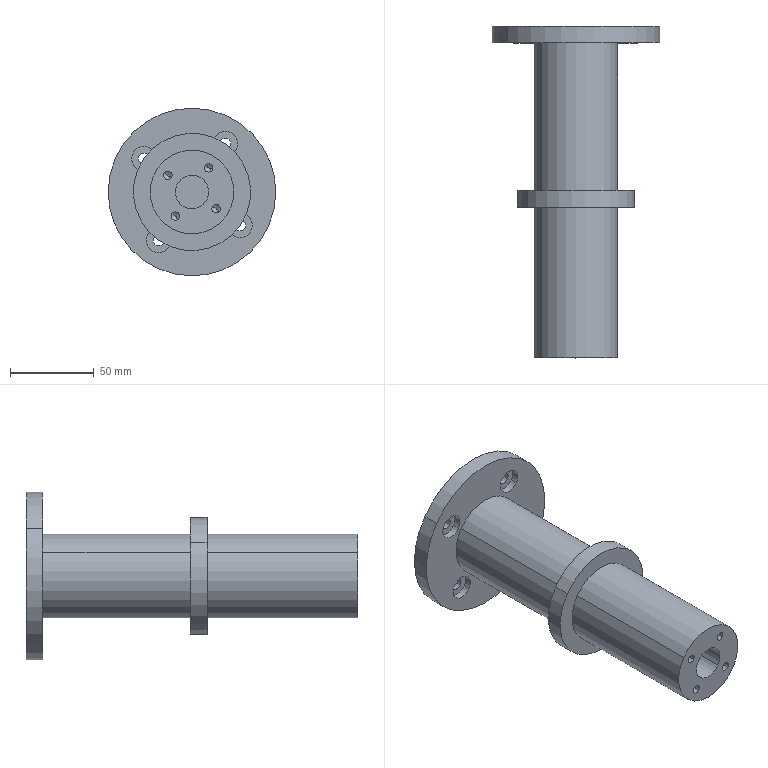Part | STEP file | M6 Tapped Hole 1 | 1 solid | 52 faces | box 100 x 198 x 100 mm | volume 452324 mm3 | cylinder 34 | plane 10 | cone 8 | commonest cylinder face diameters 5 x8 6.6 x8 14.55 x8 50 x4 20 x2 70 x2
STEP:
#1=CARTESIAN_POINT('',(-1578.988,1475.264,2948.123));
#2=VERTEX_POINT('',#1);
#3=CARTESIAN_POINT('',(-1574.875,1475.264,2945.28));
#4=VERTEX_POINT('',#3);
#5=CARTESIAN_POINT('',(-1576.931,1475.264,2946.701));
#6=DIRECTION('',(0.,-1.,0.));
#7=DIRECTION('',(0.8226,0.,-0.5686));
#8=AXIS2_PLACEMENT_3D('',#5,#6,#7);
#9=CIRCLE('',#8,2.5);
#10=EDGE_CURVE('',#2,#4,#9,.T.);
#11=ORIENTED_EDGE('',*,*,#10,.F.);
#12=CARTESIAN_POINT('',(-1578.988,1460.264,2948.123));
#13=VERTEX_POINT('',#12);
#14=CARTESIAN_POINT('',(-1578.988,1460.264,2948.123));
#15=DIRECTION('',(0.,1.,0.));
#16=VECTOR('',#15,1000.);
#17=LINE('',#14,#16);
#18=EDGE_CURVE('',#13,#2,#17,.T.);
#19=ORIENTED_EDGE('',*,*,#18,.F.);
#20=CARTESIAN_POINT('',(-1574.875,1460.264,2945.28));
#21=VERTEX_POINT('',#20);
#22=CARTESIAN_POINT('',(-1576.931,1460.264,2946.701));
#23=DIRECTION('',(0.,-1.,0.));
#24=DIRECTION('',(0.8226,0.,-0.5686));
#25=AXIS2_PLACEMENT_3D('',#22,#23,#24);
#26=CIRCLE('',#25,2.5);
#27=EDGE_CURVE('',#13,#21,#26,.T.);
#28=ORIENTED_EDGE('',*,*,#27,.T.);
#29=CARTESIAN_POINT('',(-1574.875,1460.264,2945.28));
#30=DIRECTION('',(0.,1.,0.));
#31=VECTOR('',#30,1000.);
#32=LINE('',#29,#31);
#33=EDGE_CURVE('',#21,#4,#32,.T.);
#34=ORIENTED_EDGE('',*,*,#33,.T.);
#35=EDGE_LOOP('',(#11,#19,#28,#34));
#36=FACE_OUTER_BOUND('',#35,.T.);
#37=CARTESIAN_POINT('',(-1576.931,1460.264,2946.701));
#38=DIRECTION('',(0.,-1.,0.));
#39=DIRECTION('',(-0.8226,0.,0.5686));
#40=AXIS2_PLACEMENT_3D('',#37,#38,#39);
#41=CYLINDRICAL_SURFACE('',#40,2.5);
#42=ADVANCED_FACE('',(#36),#41,.F.);
#43=CARTESIAN_POINT('',(-1576.931,1476.766,2946.701));
#44=VERTEX_POINT('',#43);
#45=CARTESIAN_POINT('',(-1574.875,1475.264,2945.28));
#46=DIRECTION('',(-0.7051,0.515,0.4874));
#47=VECTOR('',#46,1000.);
#48=LINE('',#45,#47);
#49=EDGE_CURVE('',#4,#44,#48,.T.);
#50=ORIENTED_EDGE('',*,*,#49,.T.);
#51=CARTESIAN_POINT('',(-1578.988,1475.264,2948.123));
#52=DIRECTION('',(0.7051,0.515,-0.4874));
#53=VECTOR('',#52,1000.);
#54=LINE('',#51,#53);
#55=EDGE_CURVE('',#2,#44,#54,.T.);
#56=ORIENTED_EDGE('',*,*,#55,.F.);
#57=ORIENTED_EDGE('',*,*,#10,.T.);
#58=EDGE_LOOP('',(#50,#56,#57));
#59=FACE_OUTER_BOUND('',#58,.T.);
#60=CARTESIAN_POINT('',(-1576.931,1475.264,2946.701));
#61=DIRECTION('',(0.,-1.,0.));
#62=DIRECTION('',(-0.8226,0.,0.5686));
#63=AXIS2_PLACEMENT_3D('',#60,#61,#62);
#64=CONICAL_SURFACE('',#63,2.5,1.03);
#65=ADVANCED_FACE('',(#59),#64,.F.);
#66=CARTESIAN_POINT('',(-1554.641,1475.264,2952.568));
#67=VERTEX_POINT('',#66);
#68=CARTESIAN_POINT('',(-1550.528,1475.264,2949.725));
#69=VERTEX_POINT('',#68);
#70=CARTESIAN_POINT('',(-1552.585,1475.264,2951.146));
#71=DIRECTION('',(0.,-1.,0.));
#72=DIRECTION('',(0.8226,0.,-0.5686));
#73=AXIS2_PLACEMENT_3D('',#70,#71,#72);
#74=CIRCLE('',#73,2.5);
#75=EDGE_CURVE('',#67,#69,#74,.T.);
#76=ORIENTED_EDGE('',*,*,#75,.F.);
#77=CARTESIAN_POINT('',(-1554.641,1460.264,2952.568));
#78=VERTEX_POINT('',#77);
#79=CARTESIAN_POINT('',(-1554.641,1460.264,2952.568));
#80=DIRECTION('',(0.,1.,0.));
#81=VECTOR('',#80,1000.);
#82=LINE('',#79,#81);
#83=EDGE_CURVE('',#78,#67,#82,.T.);
#84=ORIENTED_EDGE('',*,*,#83,.F.);
#85=CARTESIAN_POINT('',(-1550.528,1460.264,2949.725));
#86=VERTEX_POINT('',#85);
#87=CARTESIAN_POINT('',(-1552.585,1460.264,2951.146));
#88=DIRECTION('',(0.,-1.,0.));
#89=DIRECTION('',(0.8226,0.,-0.5686));
#90=AXIS2_PLACEMENT_3D('',#87,#88,#89);
#91=CIRCLE('',#90,2.5);
#92=EDGE_CURVE('',#78,#86,#91,.T.);
#93=ORIENTED_EDGE('',*,*,#92,.T.);
#94=CARTESIAN_POINT('',(-1550.528,1460.264,2949.725));
#95=DIRECTION('',(0.,1.,0.));
#96=VECTOR('',#95,1000.);
#97=LINE('',#94,#96);
#98=EDGE_CURVE('',#86,#69,#97,.T.);
#99=ORIENTED_EDGE('',*,*,#98,.T.);
#100=EDGE_LOOP('',(#76,#84,#93,#99));
#101=FACE_OUTER_BOUND('',#100,.T.);
#102=CARTESIAN_POINT('',(-1552.585,1460.264,2951.146));
#103=DIRECTION('',(0.,-1.,0.));
#104=DIRECTION('',(-0.8226,0.,0.5686));
#105=AXIS2_PLACEMENT_3D('',#102,#103,#104);
#106=CYLINDRICAL_SURFACE('',#105,2.5);
#107=ADVANCED_FACE('',(#101),#106,.F.);
#108=CARTESIAN_POINT('',(-1552.585,1476.766,2951.146));
#109=VERTEX_POINT('',#108);
#110=CARTESIAN_POINT('',(-1550.528,1475.264,2949.725));
#111=DIRECTION('',(-0.7051,0.515,0.4874));
#112=VECTOR('',#111,1000.);
#113=LINE('',#110,#112);
#114=EDGE_CURVE('',#69,#109,#113,.T.);
#115=ORIENTED_EDGE('',*,*,#114,.T.);
#116=CARTESIAN_POINT('',(-1554.641,1475.264,2952.568));
#117=DIRECTION('',(0.7051,0.515,-0.4874));
#118=VECTOR('',#117,1000.);
#119=LINE('',#116,#118);
#120=EDGE_CURVE('',#67,#109,#119,.T.);
#121=ORIENTED_EDGE('',*,*,#120,.F.);
#122=ORIENTED_EDGE('',*,*,#75,.T.);
#123=EDGE_LOOP('',(#115,#121,#122));
#124=FACE_OUTER_BOUND('',#123,.T.);
#125=CARTESIAN_POINT('',(-1552.585,1475.264,2951.146));
#126=DIRECTION('',(0.,-1.,0.));
#127=DIRECTION('',(-0.8226,0.,0.5686));
#128=AXIS2_PLACEMENT_3D('',#125,#126,#127);
#129=CONICAL_SURFACE('',#128,2.5,1.03);
#130=ADVANCED_FACE('',(#124),#129,.F.);
#131=CARTESIAN_POINT('',(-1550.196,1475.264,2928.222));
#132=VERTEX_POINT('',#131);
#133=CARTESIAN_POINT('',(-1546.083,1475.264,2925.378));
#134=VERTEX_POINT('',#133);
#135=CARTESIAN_POINT('',(-1548.14,1475.264,2926.8));
#136=DIRECTION('',(0.,-1.,0.));
#137=DIRECTION('',(0.8226,0.,-0.5686));
#138=AXIS2_PLACEMENT_3D('',#135,#136,#137);
#139=CIRCLE('',#138,2.5);
#140=EDGE_CURVE('',#132,#134,#139,.T.);
#141=ORIENTED_EDGE('',*,*,#140,.F.);
#142=CARTESIAN_POINT('',(-1550.196,1460.264,2928.222));
#143=VERTEX_POINT('',#142);
#144=CARTESIAN_POINT('',(-1550.196,1460.264,2928.222));
#145=DIRECTION('',(0.,1.,0.));
#146=VECTOR('',#145,1000.);
#147=LINE('',#144,#146);
#148=EDGE_CURVE('',#143,#132,#147,.T.);
#149=ORIENTED_EDGE('',*,*,#148,.F.);
#150=CARTESIAN_POINT('',(-1546.083,1460.264,2925.378));
#151=VERTEX_POINT('',#150);
#152=CARTESIAN_POINT('',(-1548.14,1460.264,2926.8));
#153=DIRECTION('',(0.,-1.,0.));
#154=DIRECTION('',(0.8226,0.,-0.5686));
#155=AXIS2_PLACEMENT_3D('',#152,#153,#154);
#156=CIRCLE('',#155,2.5);
#157=EDGE_CURVE('',#143,#151,#156,.T.);
#158=ORIENTED_EDGE('',*,*,#157,.T.);
#159=CARTESIAN_POINT('',(-1546.083,1460.264,2925.378));
#160=DIRECTION('',(0.,1.,0.));
#161=VECTOR('',#160,1000.);
#162=LINE('',#159,#161);
#163=EDGE_CURVE('',#151,#134,#162,.T.);
#164=ORIENTED_EDGE('',*,*,#163,.T.);
#165=EDGE_LOOP('',(#141,#149,#158,#164));
#166=FACE_OUTER_BOUND('',#165,.T.);
#167=CARTESIAN_POINT('',(-1548.14,1460.264,2926.8));
#168=DIRECTION('',(0.,-1.,0.));
#169=DIRECTION('',(-0.8226,0.,0.5686));
#170=AXIS2_PLACEMENT_3D('',#167,#168,#169);
#171=CYLINDRICAL_SURFACE('',#170,2.5);
#172=ADVANCED_FACE('',(#166),#171,.F.);
#173=CARTESIAN_POINT('',(-1548.14,1476.766,2926.8));
#174=VERTEX_POINT('',#173);
#175=CARTESIAN_POINT('',(-1546.083,1475.264,2925.378));
#176=DIRECTION('',(-0.7051,0.515,0.4874));
#177=VECTOR('',#176,1000.);
#178=LINE('',#175,#177);
#179=EDGE_CURVE('',#134,#174,#178,.T.);
#180=ORIENTED_EDGE('',*,*,#179,.T.);
#181=CARTESIAN_POINT('',(-1550.196,1475.264,2928.222));
#182=DIRECTION('',(0.7051,0.515,-0.4874));
#183=VECTOR('',#182,1000.);
#184=LINE('',#181,#183);
#185=EDGE_CURVE('',#132,#174,#184,.T.);
#186=ORIENTED_EDGE('',*,*,#185,.F.);
#187=ORIENTED_EDGE('',*,*,#140,.T.);
#188=EDGE_LOOP('',(#180,#186,#187));
#189=FACE_OUTER_BOUND('',#188,.T.);
#190=CARTESIAN_POINT('',(-1548.14,1475.264,2926.8));
#191=DIRECTION('',(0.,-1.,0.));
#192=DIRECTION('',(-0.8226,0.,0.5686));
#193=AXIS2_PLACEMENT_3D('',#190,#191,#192);
#194=CONICAL_SURFACE('',#193,2.5,1.03);
#195=ADVANCED_FACE('',(#189),#194,.F.);
#196=CARTESIAN_POINT('',(-1574.543,1475.264,2923.777));
#197=VERTEX_POINT('',#196);
#198=CARTESIAN_POINT('',(-1570.43,1475.264,2920.934));
#199=VERTEX_POINT('',#198);
#200=CARTESIAN_POINT('',(-1572.486,1475.264,2922.355));
#201=DIRECTION('',(0.,-1.,0.));
#202=DIRECTION('',(0.8226,0.,-0.5686));
#203=AXIS2_PLACEMENT_3D('',#200,#201,#202);
#204=CIRCLE('',#203,2.5);
#205=EDGE_CURVE('',#197,#199,#204,.T.);
#206=ORIENTED_EDGE('',*,*,#205,.F.);
#207=CARTESIAN_POINT('',(-1574.543,1460.264,2923.777));
#208=VERTEX_POINT('',#207);
#209=CARTESIAN_POINT('',(-1574.543,1460.264,2923.777));
#210=DIRECTION('',(0.,1.,0.));
#211=VECTOR('',#210,1000.);
#212=LINE('',#209,#211);
#213=EDGE_CURVE('',#208,#197,#212,.T.);
#214=ORIENTED_EDGE('',*,*,#213,.F.);
#215=CARTESIAN_POINT('',(-1570.43,1460.264,2920.934));
#216=VERTEX_POINT('',#215);
#217=CARTESIAN_POINT('',(-1572.486,1460.264,2922.355));
#218=DIRECTION('',(0.,-1.,0.));
#219=DIRECTION('',(0.8226,0.,-0.5686));
#220=AXIS2_PLACEMENT_3D('',#217,#218,#219);
#221=CIRCLE('',#220,2.5);
#222=EDGE_CURVE('',#208,#216,#221,.T.);
#223=ORIENTED_EDGE('',*,*,#222,.T.);
#224=CARTESIAN_POINT('',(-1570.43,1460.264,2920.934));
#225=DIRECTION('',(0.,1.,0.));
#226=VECTOR('',#225,1000.);
#227=LINE('',#224,#226);
#228=EDGE_CURVE('',#216,#199,#227,.T.);
#229=ORIENTED_EDGE('',*,*,#228,.T.);
#230=EDGE_LOOP('',(#206,#214,#223,#229));
#231=FACE_OUTER_BOUND('',#230,.T.);
#232=CARTESIAN_POINT('',(-1572.486,1460.264,2922.355));
#233=DIRECTION('',(0.,-1.,0.));
#234=DIRECTION('',(-0.8226,0.,0.5686));
#235=AXIS2_PLACEMENT_3D('',#232,#233,#234);
#236=CYLINDRICAL_SURFACE('',#235,2.5);
#237=ADVANCED_FACE('',(#231),#236,.F.);
#238=CARTESIAN_POINT('',(-1572.486,1476.766,2922.355));
#239=VERTEX_POINT('',#238);
#240=CARTESIAN_POINT('',(-1570.43,1475.264,2920.934));
#241=DIRECTION('',(-0.7051,0.515,0.4874));
#242=VECTOR('',#241,1000.);
#243=LINE('',#240,#242);
#244=EDGE_CURVE('',#199,#239,#243,.T.);
#245=ORIENTED_EDGE('',*,*,#244,.T.);
#246=CARTESIAN_POINT('',(-1574.543,1475.264,2923.777));
#247=DIRECTION('',(0.7051,0.515,-0.4874));
#248=VECTOR('',#247,1000.);
#249=LINE('',#246,#248);
#250=EDGE_CURVE('',#197,#239,#249,.T.);
#251=ORIENTED_EDGE('',*,*,#250,.F.);
#252=ORIENTED_EDGE('',*,*,#205,.T.);
#253=EDGE_LOOP('',(#245,#251,#252));
#254=FACE_OUTER_BOUND('',#253,.T.);
#255=CARTESIAN_POINT('',(-1572.486,1475.264,2922.355));
#256=DIRECTION('',(0.,-1.,0.));
#257=DIRECTION('',(-0.8226,0.,0.5686));
#258=AXIS2_PLACEMENT_3D('',#255,#256,#257);
#259=CONICAL_SURFACE('',#258,2.5,1.03);
#260=ADVANCED_FACE('',(#254),#259,.F.);
#261=CARTESIAN_POINT('',(-1570.762,1490.264,2942.437));
#262=VERTEX_POINT('',#261);
#263=CARTESIAN_POINT('',(-1554.309,1490.264,2931.065));
#264=VERTEX_POINT('',#263);
#265=CARTESIAN_POINT('',(-1562.535,1490.264,2936.751));
#266=DIRECTION('',(0.,-1.,0.));
#267=DIRECTION('',(0.8226,0.,-0.5686));
#268=AXIS2_PLACEMENT_3D('',#265,#266,#267);
#269=CIRCLE('',#268,10.);
#270=EDGE_CURVE('',#262,#264,#269,.T.);
#271=ORIENTED_EDGE('',*,*,#270,.F.);
#272=CARTESIAN_POINT('',(-1570.762,1460.264,2942.437));
#273=VERTEX_POINT('',#272);
#274=CARTESIAN_POINT('',(-1570.762,1490.264,2942.437));
#275=DIRECTION('',(0.,1.,0.));
#276=VECTOR('',#275,1000.);
#277=LINE('',#274,#276);
#278=EDGE_CURVE('',#273,#262,#277,.T.);
#279=ORIENTED_EDGE('',*,*,#278,.F.);
#280=CARTESIAN_POINT('',(-1554.309,1460.264,2931.065));
#281=VERTEX_POINT('',#280);
#282=CARTESIAN_POINT('',(-1562.535,1460.264,2936.751));
#283=DIRECTION('',(0.,-1.,0.));
#284=DIRECTION('',(0.8226,0.,-0.5686));
#285=AXIS2_PLACEMENT_3D('',#282,#283,#284);
#286=CIRCLE('',#285,10.);
#287=EDGE_CURVE('',#273,#281,#286,.T.);
#288=ORIENTED_EDGE('',*,*,#287,.T.);
#289=CARTESIAN_POINT('',(-1554.309,1490.264,2931.065));
#290=DIRECTION('',(0.,1.,0.));
#291=VECTOR('',#290,1000.);
#292=LINE('',#289,#291);
#293=EDGE_CURVE('',#281,#264,#292,.T.);
#294=ORIENTED_EDGE('',*,*,#293,.T.);
#295=EDGE_LOOP('',(#271,#279,#288,#294));
#296=FACE_OUTER_BOUND('',#295,.T.);
#297=CARTESIAN_POINT('',(-1562.535,1490.264,2936.751));
#298=DIRECTION('',(0.,-1.,0.));
#299=DIRECTION('',(-0.8226,0.,0.5686));
#300=AXIS2_PLACEMENT_3D('',#297,#298,#299);
#301=CYLINDRICAL_SURFACE('',#300,10.);
#302=ADVANCED_FACE('',(#296),#301,.F.);
#303=CARTESIAN_POINT('',(-1541.97,1550.264,2922.535));
#304=VERTEX_POINT('',#303);
#305=CARTESIAN_POINT('',(-1583.101,1550.264,2950.966));
#306=VERTEX_POINT('',#305);
#307=CARTESIAN_POINT('',(-1562.535,1550.264,2936.751));
#308=DIRECTION('',(0.,-1.,0.));
#309=DIRECTION('',(0.8226,0.,-0.5686));
#310=AXIS2_PLACEMENT_3D('',#307,#308,#309);
#311=CIRCLE('',#310,25.);
#312=EDGE_CURVE('',#304,#306,#311,.T.);
#313=ORIENTED_EDGE('',*,*,#312,.T.);
#314=CARTESIAN_POINT('',(-1583.101,1460.264,2950.966));
#315=VERTEX_POINT('',#314);
#316=CARTESIAN_POINT('',(-1583.101,1648.264,2950.966));
#317=DIRECTION('',(0.,1.,0.));
#318=VECTOR('',#317,1000.);
#319=LINE('',#316,#318);
#320=EDGE_CURVE('',#315,#306,#319,.T.);
#321=ORIENTED_EDGE('',*,*,#320,.F.);
#322=CARTESIAN_POINT('',(-1541.97,1460.264,2922.535));
#323=VERTEX_POINT('',#322);
#324=CARTESIAN_POINT('',(-1562.535,1460.264,2936.751));
#325=DIRECTION('',(0.,1.,0.));
#326=DIRECTION('',(-0.8226,0.,0.5686));
#327=AXIS2_PLACEMENT_3D('',#324,#325,#326);
#328=CIRCLE('',#327,25.);
#329=EDGE_CURVE('',#315,#323,#328,.T.);
#330=ORIENTED_EDGE('',*,*,#329,.T.);
#331=CARTESIAN_POINT('',(-1541.97,1648.264,2922.535));
#332=DIRECTION('',(0.,1.,0.));
#333=VECTOR('',#332,1000.);
#334=LINE('',#331,#333);
#335=EDGE_CURVE('',#323,#304,#334,.T.);
#336=ORIENTED_EDGE('',*,*,#335,.T.);
#337=EDGE_LOOP('',(#313,#321,#330,#336));
#338=FACE_OUTER_BOUND('',#337,.T.);
#339=CARTESIAN_POINT('',(-1562.535,1648.264,2936.751));
#340=DIRECTION('',(0.,-1.,0.));
#341=DIRECTION('',(-0.8226,0.,0.5686));
#342=AXIS2_PLACEMENT_3D('',#339,#340,#341);
#343=CYLINDRICAL_SURFACE('',#342,25.);
#344=ADVANCED_FACE('',(#338),#343,.T.);
#345=CARTESIAN_POINT('',(-1533.744,1550.264,2916.849));
#346=VERTEX_POINT('',#345);
#347=CARTESIAN_POINT('',(-1591.327,1550.264,2956.652));
#348=VERTEX_POINT('',#347);
#349=CARTESIAN_POINT('',(-1562.535,1550.264,2936.751));
#350=DIRECTION('',(0.,-1.,0.));
#351=DIRECTION('',(0.8226,0.,-0.5686));
#352=AXIS2_PLACEMENT_3D('',#349,#350,#351);
#353=CIRCLE('',#352,35.);
#354=EDGE_CURVE('',#346,#348,#353,.T.);
#355=ORIENTED_EDGE('',*,*,#354,.F.);
#356=CARTESIAN_POINT('',(-1533.744,1560.264,2916.849));
#357=VERTEX_POINT('',#356);
#358=CARTESIAN_POINT('',(-1533.744,1550.264,2916.849));
#359=DIRECTION('',(0.,1.,0.));
#360=VECTOR('',#359,1000.);
#361=LINE('',#358,#360);
#362=EDGE_CURVE('',#346,#357,#361,.T.);
#363=ORIENTED_EDGE('',*,*,#362,.T.);
#364=CARTESIAN_POINT('',(-1591.327,1560.264,2956.652));
#365=VERTEX_POINT('',#364);
#366=CARTESIAN_POINT('',(-1562.535,1560.264,2936.751));
#367=DIRECTION('',(0.,-1.,0.));
#368=DIRECTION('',(0.8226,0.,-0.5686));
#369=AXIS2_PLACEMENT_3D('',#366,#367,#368);
#370=CIRCLE('',#369,35.);
#371=EDGE_CURVE('',#357,#365,#370,.T.);
#372=ORIENTED_EDGE('',*,*,#371,.T.);
#373=CARTESIAN_POINT('',(-1591.327,1550.264,2956.652));
#374=DIRECTION('',(0.,1.,0.));
#375=VECTOR('',#374,1000.);
#376=LINE('',#373,#375);
#377=EDGE_CURVE('',#348,#365,#376,.T.);
#378=ORIENTED_EDGE('',*,*,#377,.F.);
#379=EDGE_LOOP('',(#355,#363,#372,#378));
#380=FACE_OUTER_BOUND('',#379,.T.);
#381=CARTESIAN_POINT('',(-1562.535,1550.264,2936.751));
#382=DIRECTION('',(0.,1.,0.));
#383=DIRECTION('',(0.8226,0.,-0.5686));
#384=AXIS2_PLACEMENT_3D('',#381,#382,#383);
#385=CYLINDRICAL_SURFACE('',#384,35.);
#386=ADVANCED_FACE('',(#380),#385,.T.);
#387=CARTESIAN_POINT('',(-1539.729,1652.414,2920.986));
#388=VERTEX_POINT('',#387);
#389=CARTESIAN_POINT('',(-1527.76,1652.414,2912.713));
#390=VERTEX_POINT('',#389);
#391=CARTESIAN_POINT('',(-1533.744,1652.414,2916.849));
#392=DIRECTION('',(0.,-1.,0.));
#393=DIRECTION('',(0.8226,0.,-0.5686));
#394=AXIS2_PLACEMENT_3D('',#391,#392,#393);
#395=CIRCLE('',#394,7.275);
#396=EDGE_CURVE('',#388,#390,#395,.T.);
#397=ORIENTED_EDGE('',*,*,#396,.F.);
#398=CARTESIAN_POINT('',(-1539.729,1648.264,2920.986));
#399=VERTEX_POINT('',#398);
#400=CARTESIAN_POINT('',(-1539.729,1648.264,2920.986));
#401=DIRECTION('',(0.,1.,0.));
#402=VECTOR('',#401,1000.);
#403=LINE('',#400,#402);
#404=EDGE_CURVE('',#399,#388,#403,.T.);
#405=ORIENTED_EDGE('',*,*,#404,.F.);
#406=CARTESIAN_POINT('',(-1527.76,1648.264,2912.713));
#407=VERTEX_POINT('',#406);
#408=CARTESIAN_POINT('',(-1533.744,1648.264,2916.849));
#409=DIRECTION('',(0.,-1.,0.));
#410=DIRECTION('',(0.8226,0.,-0.5686));
#411=AXIS2_PLACEMENT_3D('',#408,#409,#410);
#412=CIRCLE('',#411,7.275);
#413=EDGE_CURVE('',#399,#407,#412,.T.);
#414=ORIENTED_EDGE('',*,*,#413,.T.);
#415=CARTESIAN_POINT('',(-1527.76,1648.264,2912.713));
#416=DIRECTION('',(0.,1.,0.));
#417=VECTOR('',#416,1000.);
#418=LINE('',#415,#417);
#419=EDGE_CURVE('',#407,#390,#418,.T.);
#420=ORIENTED_EDGE('',*,*,#419,.T.);
#421=EDGE_LOOP('',(#397,#405,#414,#420));
#422=FACE_OUTER_BOUND('',#421,.T.);
#423=CARTESIAN_POINT('',(-1533.744,1648.264,2916.849));
#424=DIRECTION('',(0.,-1.,0.));
#425=DIRECTION('',(-0.8226,0.,0.5686));
#426=AXIS2_PLACEMENT_3D('',#423,#424,#425);
#427=CYLINDRICAL_SURFACE('',#426,7.275);
#428=ADVANCED_FACE('',(#422),#427,.F.);
#429=CARTESIAN_POINT('',(-1536.459,1658.264,2918.726));
#430=VERTEX_POINT('',#429);
#431=CARTESIAN_POINT('',(-1531.03,1658.264,2914.973));
#432=VERTEX_POINT('',#431);
#433=CARTESIAN_POINT('',(-1533.744,1658.264,2916.849));
#434=DIRECTION('',(0.,-1.,0.));
#435=DIRECTION('',(0.8226,0.,-0.5686));
#436=AXIS2_PLACEMENT_3D('',#433,#434,#435);
#437=CIRCLE('',#436,3.3);
#438=EDGE_CURVE('',#430,#432,#437,.T.);
#439=ORIENTED_EDGE('',*,*,#438,.F.);
#440=CARTESIAN_POINT('',(-1536.459,1652.414,2918.726));
#441=VERTEX_POINT('',#440);
#442=CARTESIAN_POINT('',(-1536.459,1648.264,2918.726));
#443=DIRECTION('',(0.,1.,0.));
#444=VECTOR('',#443,1000.);
#445=LINE('',#442,#444);
#446=EDGE_CURVE('',#441,#430,#445,.T.);
#447=ORIENTED_EDGE('',*,*,#446,.F.);
#448=CARTESIAN_POINT('',(-1531.03,1652.414,2914.973));
#449=VERTEX_POINT('',#448);
#450=CARTESIAN_POINT('',(-1533.744,1652.414,2916.849));
#451=DIRECTION('',(0.,-1.,0.));
#452=DIRECTION('',(0.8226,0.,-0.5686));
#453=AXIS2_PLACEMENT_3D('',#450,#451,#452);
#454=CIRCLE('',#453,3.3);
#455=EDGE_CURVE('',#441,#449,#454,.T.);
#456=ORIENTED_EDGE('',*,*,#455,.T.);
#457=CARTESIAN_POINT('',(-1531.03,1648.264,2914.973));
#458=DIRECTION('',(0.,1.,0.));
#459=VECTOR('',#458,1000.);
#460=LINE('',#457,#459);
#461=EDGE_CURVE('',#449,#432,#460,.T.);
#462=ORIENTED_EDGE('',*,*,#461,.T.);
#463=EDGE_LOOP('',(#439,#447,#456,#462));
#464=FACE_OUTER_BOUND('',#463,.T.);
#465=CARTESIAN_POINT('',(-1533.744,1648.264,2916.849));
#466=DIRECTION('',(0.,-1.,0.));
#467=DIRECTION('',(-0.8226,0.,0.5686));
#468=AXIS2_PLACEMENT_3D('',#465,#466,#467);
#469=CYLINDRICAL_SURFACE('',#468,3.3);
#470=ADVANCED_FACE('',(#464),#469,.F.);
#471=CARTESIAN_POINT('',(-1588.421,1652.414,2912.096));
#472=VERTEX_POINT('',#471);
#473=CARTESIAN_POINT('',(-1576.452,1652.414,2903.823));
#474=VERTEX_POINT('',#473);
#475=CARTESIAN_POINT('',(-1582.437,1652.414,2907.959));
#476=DIRECTION('',(0.,-1.,0.));
#477=DIRECTION('',(0.8226,0.,-0.5686));
#478=AXIS2_PLACEMENT_3D('',#475,#476,#477);
#479=CIRCLE('',#478,7.275);
#480=EDGE_CURVE('',#472,#474,#479,.T.);
#481=ORIENTED_EDGE('',*,*,#480,.F.);
#482=CARTESIAN_POINT('',(-1588.421,1648.264,2912.096));
#483=VERTEX_POINT('',#482);
#484=CARTESIAN_POINT('',(-1588.421,1648.264,2912.096));
#485=DIRECTION('',(0.,1.,0.));
#486=VECTOR('',#485,1000.);
#487=LINE('',#484,#486);
#488=EDGE_CURVE('',#483,#472,#487,.T.);
#489=ORIENTED_EDGE('',*,*,#488,.F.);
#490=CARTESIAN_POINT('',(-1576.452,1648.264,2903.823));
#491=VERTEX_POINT('',#490);
#492=CARTESIAN_POINT('',(-1582.437,1648.264,2907.959));
#493=DIRECTION('',(0.,-1.,0.));
#494=DIRECTION('',(0.8226,0.,-0.5686));
#495=AXIS2_PLACEMENT_3D('',#492,#493,#494);
#496=CIRCLE('',#495,7.275);
#497=EDGE_CURVE('',#483,#491,#496,.T.);
#498=ORIENTED_EDGE('',*,*,#497,.T.);
#499=CARTESIAN_POINT('',(-1576.452,1648.264,2903.823));
#500=DIRECTION('',(0.,1.,0.));
#501=VECTOR('',#500,1000.);
#502=LINE('',#499,#501);
#503=EDGE_CURVE('',#491,#474,#502,.T.);
#504=ORIENTED_EDGE('',*,*,#503,.T.);
#505=EDGE_LOOP('',(#481,#489,#498,#504));
#506=FACE_OUTER_BOUND('',#505,.T.);
#507=CARTESIAN_POINT('',(-1582.437,1648.264,2907.959));
#508=DIRECTION('',(0.,-1.,0.));
#509=DIRECTION('',(-0.8226,0.,0.5686));
#510=AXIS2_PLACEMENT_3D('',#507,#508,#509);
#511=CYLINDRICAL_SURFACE('',#510,7.275);
#512=ADVANCED_FACE('',(#506),#511,.F.);
#513=CARTESIAN_POINT('',(-1585.151,1658.264,2909.836));
#514=VERTEX_POINT('',#513);
#515=CARTESIAN_POINT('',(-1579.722,1658.264,2906.083));
#516=VERTEX_POINT('',#515);
#517=CARTESIAN_POINT('',(-1582.437,1658.264,2907.959));
#518=DIRECTION('',(0.,-1.,0.));
#519=DIRECTION('',(0.8226,0.,-0.5686));
#520=AXIS2_PLACEMENT_3D('',#517,#518,#519);
#521=CIRCLE('',#520,3.3);
#522=EDGE_CURVE('',#514,#516,#521,.T.);
#523=ORIENTED_EDGE('',*,*,#522,.F.);
#524=CARTESIAN_POINT('',(-1585.151,1652.414,2909.836));
#525=VERTEX_POINT('',#524);
#526=CARTESIAN_POINT('',(-1585.151,1648.264,2909.836));
#527=DIRECTION('',(0.,1.,0.));
#528=VECTOR('',#527,1000.);
#529=LINE('',#526,#528);
#530=EDGE_CURVE('',#525,#514,#529,.T.);
#531=ORIENTED_EDGE('',*,*,#530,.F.);
#532=CARTESIAN_POINT('',(-1579.722,1652.414,2906.083));
#533=VERTEX_POINT('',#532);
#534=CARTESIAN_POINT('',(-1582.437,1652.414,2907.959));
#535=DIRECTION('',(0.,-1.,0.));
#536=DIRECTION('',(0.8226,0.,-0.5686));
#537=AXIS2_PLACEMENT_3D('',#534,#535,#536);
#538=CIRCLE('',#537,3.3);
#539=EDGE_CURVE('',#525,#533,#538,.T.);
#540=ORIENTED_EDGE('',*,*,#539,.T.);
#541=CARTESIAN_POINT('',(-1579.722,1648.264,2906.083));
#542=DIRECTION('',(0.,1.,0.));
#543=VECTOR('',#542,1000.);
#544=LINE('',#541,#543);
#545=EDGE_CURVE('',#533,#516,#544,.T.);
#546=ORIENTED_EDGE('',*,*,#545,.T.);
#547=EDGE_LOOP('',(#523,#531,#540,#546));
#548=FACE_OUTER_BOUND('',#547,.T.);
#549=CARTESIAN_POINT('',(-1582.437,1648.264,2907.959));
#550=DIRECTION('',(0.,-1.,0.));
#551=DIRECTION('',(-0.8226,0.,0.5686));
#552=AXIS2_PLACEMENT_3D('',#549,#550,#551);
#553=CYLINDRICAL_SURFACE('',#552,3.3);
#554=ADVANCED_FACE('',(#548),#553,.F.);
#555=CARTESIAN_POINT('',(-1597.311,1652.414,2960.789));
#556=VERTEX_POINT('',#555);
#557=CARTESIAN_POINT('',(-1585.342,1652.414,2952.515));
#558=VERTEX_POINT('',#557);
#559=CARTESIAN_POINT('',(-1591.327,1652.414,2956.652));
#560=DIRECTION('',(0.,-1.,0.));
#561=DIRECTION('',(0.8226,0.,-0.5686));
#562=AXIS2_PLACEMENT_3D('',#559,#560,#561);
#563=CIRCLE('',#562,7.275);
#564=EDGE_CURVE('',#556,#558,#563,.T.);
#565=ORIENTED_EDGE('',*,*,#564,.F.);
#566=CARTESIAN_POINT('',(-1597.311,1648.264,2960.789));
#567=VERTEX_POINT('',#566);
#568=CARTESIAN_POINT('',(-1597.311,1648.264,2960.789));
#569=DIRECTION('',(0.,1.,0.));
#570=VECTOR('',#569,1000.);
#571=LINE('',#568,#570);
#572=EDGE_CURVE('',#567,#556,#571,.T.);
#573=ORIENTED_EDGE('',*,*,#572,.F.);
#574=CARTESIAN_POINT('',(-1585.342,1648.264,2952.515));
#575=VERTEX_POINT('',#574);
#576=CARTESIAN_POINT('',(-1591.327,1648.264,2956.652));
#577=DIRECTION('',(0.,-1.,0.));
#578=DIRECTION('',(0.8226,0.,-0.5686));
#579=AXIS2_PLACEMENT_3D('',#576,#577,#578);
#580=CIRCLE('',#579,7.275);
#581=EDGE_CURVE('',#567,#575,#580,.T.);
#582=ORIENTED_EDGE('',*,*,#581,.T.);
#583=CARTESIAN_POINT('',(-1585.342,1648.264,2952.515));
#584=DIRECTION('',(0.,1.,0.));
#585=VECTOR('',#584,1000.);
#586=LINE('',#583,#585);
#587=EDGE_CURVE('',#575,#558,#586,.T.);
#588=ORIENTED_EDGE('',*,*,#587,.T.);
#589=EDGE_LOOP('',(#565,#573,#582,#588));
#590=FACE_OUTER_BOUND('',#589,.T.);
#591=CARTESIAN_POINT('',(-1591.327,1648.264,2956.652));
#592=DIRECTION('',(0.,-1.,0.));
#593=DIRECTION('',(-0.8226,0.,0.5686));
#594=AXIS2_PLACEMENT_3D('',#591,#592,#593);
#595=CYLINDRICAL_SURFACE('',#594,7.275);
#596=ADVANCED_FACE('',(#590),#595,.F.);
#597=CARTESIAN_POINT('',(-1594.041,1658.264,2958.528));
#598=VERTEX_POINT('',#597);
#599=CARTESIAN_POINT('',(-1588.612,1658.264,2954.776));
#600=VERTEX_POINT('',#599);
#601=CARTESIAN_POINT('',(-1591.327,1658.264,2956.652));
#602=DIRECTION('',(0.,-1.,0.));
#603=DIRECTION('',(0.8226,0.,-0.5686));
#604=AXIS2_PLACEMENT_3D('',#601,#602,#603);
#605=CIRCLE('',#604,3.3);
#606=EDGE_CURVE('',#598,#600,#605,.T.);
#607=ORIENTED_EDGE('',*,*,#606,.F.);
#608=CARTESIAN_POINT('',(-1594.041,1652.414,2958.528));
#609=VERTEX_POINT('',#608);
#610=CARTESIAN_POINT('',(-1594.041,1648.264,2958.528));
#611=DIRECTION('',(0.,1.,0.));
#612=VECTOR('',#611,1000.);
#613=LINE('',#610,#612);
#614=EDGE_CURVE('',#609,#598,#613,.T.);
#615=ORIENTED_EDGE('',*,*,#614,.F.);
#616=CARTESIAN_POINT('',(-1588.612,1652.414,2954.776));
#617=VERTEX_POINT('',#616);
#618=CARTESIAN_POINT('',(-1591.327,1652.414,2956.652));
#619=DIRECTION('',(0.,-1.,0.));
#620=DIRECTION('',(0.8226,0.,-0.5686));
#621=AXIS2_PLACEMENT_3D('',#618,#619,#620);
#622=CIRCLE('',#621,3.3);
#623=EDGE_CURVE('',#609,#617,#622,.T.);
#624=ORIENTED_EDGE('',*,*,#623,.T.);
#625=CARTESIAN_POINT('',(-1588.612,1648.264,2954.776));
#626=DIRECTION('',(0.,1.,0.));
#627=VECTOR('',#626,1000.);
#628=LINE('',#625,#627);
#629=EDGE_CURVE('',#617,#600,#628,.T.);
#630=ORIENTED_EDGE('',*,*,#629,.T.);
#631=EDGE_LOOP('',(#607,#615,#624,#630));
#632=FACE_OUTER_BOUND('',#631,.T.);
#633=CARTESIAN_POINT('',(-1591.327,1648.264,2956.652));
#634=DIRECTION('',(0.,-1.,0.));
#635=DIRECTION('',(-0.8226,0.,0.5686));
#636=AXIS2_PLACEMENT_3D('',#633,#634,#635);
#637=CYLINDRICAL_SURFACE('',#636,3.3);
#638=ADVANCED_FACE('',(#632),#637,.F.);
#639=CARTESIAN_POINT('',(-1548.619,1652.414,2969.679));
#640=VERTEX_POINT('',#639);
#641=CARTESIAN_POINT('',(-1536.65,1652.414,2961.405));
#642=VERTEX_POINT('',#641);
#643=CARTESIAN_POINT('',(-1542.634,1652.414,2965.542));
#644=DIRECTION('',(0.,-1.,0.));
#645=DIRECTION('',(0.8226,0.,-0.5686));
#646=AXIS2_PLACEMENT_3D('',#643,#644,#645);
#647=CIRCLE('',#646,7.275);
#648=EDGE_CURVE('',#640,#642,#647,.T.);
#649=ORIENTED_EDGE('',*,*,#648,.F.);
#650=CARTESIAN_POINT('',(-1548.619,1648.264,2969.679));
#651=VERTEX_POINT('',#650);
#652=CARTESIAN_POINT('',(-1548.619,1648.264,2969.679));
#653=DIRECTION('',(0.,1.,0.));
#654=VECTOR('',#653,1000.);
#655=LINE('',#652,#654);
#656=EDGE_CURVE('',#651,#640,#655,.T.);
#657=ORIENTED_EDGE('',*,*,#656,.F.);
#658=CARTESIAN_POINT('',(-1536.65,1648.264,2961.405));
#659=VERTEX_POINT('',#658);
#660=CARTESIAN_POINT('',(-1542.634,1648.264,2965.542));
#661=DIRECTION('',(0.,-1.,0.));
#662=DIRECTION('',(0.8226,0.,-0.5686));
#663=AXIS2_PLACEMENT_3D('',#660,#661,#662);
#664=CIRCLE('',#663,7.275);
#665=EDGE_CURVE('',#651,#659,#664,.T.);
#666=ORIENTED_EDGE('',*,*,#665,.T.);
#667=CARTESIAN_POINT('',(-1536.65,1648.264,2961.405));
#668=DIRECTION('',(0.,1.,0.));
#669=VECTOR('',#668,1000.);
#670=LINE('',#667,#669);
#671=EDGE_CURVE('',#659,#642,#670,.T.);
#672=ORIENTED_EDGE('',*,*,#671,.T.);
#673=EDGE_LOOP('',(#649,#657,#666,#672));
#674=FACE_OUTER_BOUND('',#673,.T.);
#675=CARTESIAN_POINT('',(-1542.634,1648.264,2965.542));
#676=DIRECTION('',(0.,-1.,0.));
#677=DIRECTION('',(-0.8226,0.,0.5686));
#678=AXIS2_PLACEMENT_3D('',#675,#676,#677);
#679=CYLINDRICAL_SURFACE('',#678,7.275);
#680=ADVANCED_FACE('',(#674),#679,.F.);
#681=CARTESIAN_POINT('',(-1545.349,1658.264,2967.418));
#682=VERTEX_POINT('',#681);
#683=CARTESIAN_POINT('',(-1539.919,1658.264,2963.666));
#684=VERTEX_POINT('',#683);
#685=CARTESIAN_POINT('',(-1542.634,1658.264,2965.542));
#686=DIRECTION('',(0.,-1.,0.));
#687=DIRECTION('',(0.8226,0.,-0.5686));
#688=AXIS2_PLACEMENT_3D('',#685,#686,#687);
#689=CIRCLE('',#688,3.3);
#690=EDGE_CURVE('',#682,#684,#689,.T.);
#691=ORIENTED_EDGE('',*,*,#690,.F.);
#692=CARTESIAN_POINT('',(-1545.349,1652.414,2967.418));
#693=VERTEX_POINT('',#692);
#694=CARTESIAN_POINT('',(-1545.349,1648.264,2967.418));
#695=DIRECTION('',(0.,1.,0.));
#696=VECTOR('',#695,1000.);
#697=LINE('',#694,#696);
#698=EDGE_CURVE('',#693,#682,#697,.T.);
#699=ORIENTED_EDGE('',*,*,#698,.F.);
#700=CARTESIAN_POINT('',(-1539.919,1652.414,2963.666));
#701=VERTEX_POINT('',#700);
#702=CARTESIAN_POINT('',(-1542.634,1652.414,2965.542));
#703=DIRECTION('',(0.,-1.,0.));
#704=DIRECTION('',(0.8226,0.,-0.5686));
#705=AXIS2_PLACEMENT_3D('',#702,#703,#704);
#706=CIRCLE('',#705,3.3);
#707=EDGE_CURVE('',#693,#701,#706,.T.);
#708=ORIENTED_EDGE('',*,*,#707,.T.);
#709=CARTESIAN_POINT('',(-1539.919,1648.264,2963.666));
#710=DIRECTION('',(0.,1.,0.));
#711=VECTOR('',#710,1000.);
#712=LINE('',#709,#711);
#713=EDGE_CURVE('',#701,#684,#712,.T.);
#714=ORIENTED_EDGE('',*,*,#713,.T.);
#715=EDGE_LOOP('',(#691,#699,#708,#714));
#716=FACE_OUTER_BOUND('',#715,.T.);
#717=CARTESIAN_POINT('',(-1542.634,1648.264,2965.542));
#718=DIRECTION('',(0.,-1.,0.));
#719=DIRECTION('',(-0.8226,0.,0.5686));
#720=AXIS2_PLACEMENT_3D('',#717,#718,#719);
#721=CYLINDRICAL_SURFACE('',#720,3.3);
#722=ADVANCED_FACE('',(#716),#721,.F.);
#723=CARTESIAN_POINT('',(-1603.666,1658.264,2965.181));
#724=VERTEX_POINT('',#723);
#725=CARTESIAN_POINT('',(-1521.405,1658.264,2908.32));
#726=VERTEX_POINT('',#725);
#727=CARTESIAN_POINT('',(-1562.535,1658.264,2936.751));
#728=DIRECTION('',(0.,1.,0.));
#729=DIRECTION('',(-0.8226,0.,0.5686));
#730=AXIS2_PLACEMENT_3D('',#727,#728,#729);
#731=CIRCLE('',#730,50.);
#732=EDGE_CURVE('',#724,#726,#731,.T.);
#733=ORIENTED_EDGE('',*,*,#732,.F.);
#734=CARTESIAN_POINT('',(-1603.666,1648.264,2965.181));
#735=VERTEX_POINT('',#734);
#736=CARTESIAN_POINT('',(-1603.666,1658.264,2965.181));
#737=DIRECTION('',(0.,1.,0.));
#738=VECTOR('',#737,1000.);
#739=LINE('',#736,#738);
#740=EDGE_CURVE('',#735,#724,#739,.T.);
#741=ORIENTED_EDGE('',*,*,#740,.F.);
#742=CARTESIAN_POINT('',(-1521.405,1648.264,2908.32));
#743=VERTEX_POINT('',#742);
#744=CARTESIAN_POINT('',(-1562.535,1648.264,2936.751));
#745=DIRECTION('',(0.,1.,0.));
#746=DIRECTION('',(-0.8226,0.,0.5686));
#747=AXIS2_PLACEMENT_3D('',#744,#745,#746);
#748=CIRCLE('',#747,50.);
#749=EDGE_CURVE('',#735,#743,#748,.T.);
#750=ORIENTED_EDGE('',*,*,#749,.T.);
#751=CARTESIAN_POINT('',(-1521.405,1658.264,2908.32));
#752=DIRECTION('',(0.,1.,0.));
#753=VECTOR('',#752,1000.);
#754=LINE('',#751,#753);
#755=EDGE_CURVE('',#743,#726,#754,.T.);
#756=ORIENTED_EDGE('',*,*,#755,.T.);
#757=EDGE_LOOP('',(#733,#741,#750,#756));
#758=FACE_OUTER_BOUND('',#757,.T.);
#759=CARTESIAN_POINT('',(-1562.535,1658.264,2936.751));
#760=DIRECTION('',(0.,-1.,0.));
#761=DIRECTION('',(-0.8226,0.,0.5686));
#762=AXIS2_PLACEMENT_3D('',#759,#760,#761);
#763=CYLINDRICAL_SURFACE('',#762,50.);
#764=ADVANCED_FACE('',(#758),#763,.T.);
#765=CARTESIAN_POINT('',(-1583.101,1648.264,2950.966));
#766=VERTEX_POINT('',#765);
#767=CARTESIAN_POINT('',(-1541.97,1648.264,2922.535));
#768=VERTEX_POINT('',#767);
#769=CARTESIAN_POINT('',(-1562.535,1648.264,2936.751));
#770=DIRECTION('',(0.,1.,0.));
#771=DIRECTION('',(-0.8226,0.,0.5686));
#772=AXIS2_PLACEMENT_3D('',#769,#770,#771);
#773=CIRCLE('',#772,25.);
#774=EDGE_CURVE('',#766,#768,#773,.T.);
#775=ORIENTED_EDGE('',*,*,#774,.F.);
#776=CARTESIAN_POINT('',(-1583.101,1560.264,2950.966));
#777=VERTEX_POINT('',#776);
#778=CARTESIAN_POINT('',(-1583.101,1648.264,2950.966));
#779=DIRECTION('',(0.,1.,0.));
#780=VECTOR('',#779,1000.);
#781=LINE('',#778,#780);
#782=EDGE_CURVE('',#777,#766,#781,.T.);
#783=ORIENTED_EDGE('',*,*,#782,.F.);
#784=CARTESIAN_POINT('',(-1541.97,1560.264,2922.535));
#785=VERTEX_POINT('',#784);
#786=CARTESIAN_POINT('',(-1562.535,1560.264,2936.751));
#787=DIRECTION('',(0.,-1.,0.));
#788=DIRECTION('',(0.8226,0.,-0.5686));
#789=AXIS2_PLACEMENT_3D('',#786,#787,#788);
#790=CIRCLE('',#789,25.);
#791=EDGE_CURVE('',#785,#777,#790,.T.);
#792=ORIENTED_EDGE('',*,*,#791,.F.);
#793=CARTESIAN_POINT('',(-1541.97,1648.264,2922.535));
#794=DIRECTION('',(0.,1.,0.));
#795=VECTOR('',#794,1000.);
#796=LINE('',#793,#795);
#797=EDGE_CURVE('',#785,#768,#796,.T.);
#798=ORIENTED_EDGE('',*,*,#797,.T.);
#799=EDGE_LOOP('',(#775,#783,#792,#798));
#800=FACE_OUTER_BOUND('',#799,.T.);
#801=CARTESIAN_POINT('',(-1562.535,1648.264,2936.751));
#802=DIRECTION('',(0.,-1.,0.));
#803=DIRECTION('',(-0.8226,0.,0.5686));
#804=AXIS2_PLACEMENT_3D('',#801,#802,#803);
#805=CYLINDRICAL_SURFACE('',#804,25.);
#806=ADVANCED_FACE('',(#800),#805,.T.);
#807=ORIENTED_EDGE('',*,*,#782,.T.);
#808=CARTESIAN_POINT('',(-1562.535,1648.264,2936.751));
#809=DIRECTION('',(0.,1.,0.));
#810=DIRECTION('',(-0.8226,0.,0.5686));
#811=AXIS2_PLACEMENT_3D('',#808,#809,#810);
#812=CIRCLE('',#811,25.);
#813=EDGE_CURVE('',#768,#766,#812,.T.);
#814=ORIENTED_EDGE('',*,*,#813,.F.);
#815=ORIENTED_EDGE('',*,*,#797,.F.);
#816=CARTESIAN_POINT('',(-1562.535,1560.264,2936.751));
#817=DIRECTION('',(0.,-1.,0.));
#818=DIRECTION('',(0.8226,0.,-0.5686));
#819=AXIS2_PLACEMENT_3D('',#816,#817,#818);
#820=CIRCLE('',#819,25.);
#821=EDGE_CURVE('',#777,#785,#820,.T.);
#822=ORIENTED_EDGE('',*,*,#821,.F.);
#823=EDGE_LOOP('',(#807,#814,#815,#822));
#824=FACE_OUTER_BOUND('',#823,.T.);
#825=CARTESIAN_POINT('',(-1562.535,1648.264,2936.751));
#826=DIRECTION('',(0.,-1.,0.));
#827=DIRECTION('',(-0.8226,0.,0.5686));
#828=AXIS2_PLACEMENT_3D('',#825,#826,#827);
#829=CYLINDRICAL_SURFACE('',#828,25.);
#830=ADVANCED_FACE('',(#824),#829,.T.);
#831=CARTESIAN_POINT('',(-1533.744,1648.264,2916.849));
#832=DIRECTION('',(0.,-1.,0.));
#833=DIRECTION('',(0.8226,0.,-0.5686));
#834=AXIS2_PLACEMENT_3D('',#831,#832,#833);
#835=CIRCLE('',#834,7.275);
#836=EDGE_CURVE('',#407,#399,#835,.T.);
#837=ORIENTED_EDGE('',*,*,#836,.F.);
#838=ORIENTED_EDGE('',*,*,#413,.F.);
#839=EDGE_LOOP('',(#837,#838));
#840=FACE_BOUND('',#839,.T.);
#841=CARTESIAN_POINT('',(-1582.437,1648.264,2907.959));
#842=DIRECTION('',(0.,-1.,0.));
#843=DIRECTION('',(0.8226,0.,-0.5686));
#844=AXIS2_PLACEMENT_3D('',#841,#842,#843);
#845=CIRCLE('',#844,7.275);
#846=EDGE_CURVE('',#491,#483,#845,.T.);
#847=ORIENTED_EDGE('',*,*,#846,.F.);
#848=ORIENTED_EDGE('',*,*,#497,.F.);
#849=EDGE_LOOP('',(#847,#848));
#850=FACE_BOUND('',#849,.T.);
#851=CARTESIAN_POINT('',(-1591.327,1648.264,2956.652));
#852=DIRECTION('',(0.,-1.,0.));
#853=DIRECTION('',(0.8226,0.,-0.5686));
#854=AXIS2_PLACEMENT_3D('',#851,#852,#853);
#855=CIRCLE('',#854,7.275);
#856=EDGE_CURVE('',#575,#567,#855,.T.);
#857=ORIENTED_EDGE('',*,*,#856,.F.);
#858=ORIENTED_EDGE('',*,*,#581,.F.);
#859=EDGE_LOOP('',(#857,#858));
#860=FACE_BOUND('',#859,.T.);
#861=CARTESIAN_POINT('',(-1542.634,1648.264,2965.542));
#862=DIRECTION('',(0.,-1.,0.));
#863=DIRECTION('',(0.8226,0.,-0.5686));
#864=AXIS2_PLACEMENT_3D('',#861,#862,#863);
#865=CIRCLE('',#864,7.275);
#866=EDGE_CURVE('',#659,#651,#865,.T.);
#867=ORIENTED_EDGE('',*,*,#866,.F.);
#868=ORIENTED_EDGE('',*,*,#665,.F.);
#869=EDGE_LOOP('',(#867,#868));
#870=FACE_BOUND('',#869,.T.);
#871=CARTESIAN_POINT('',(-1562.535,1648.264,2936.751));
#872=DIRECTION('',(0.,1.,0.));
#873=DIRECTION('',(-0.8226,0.,0.5686));
#874=AXIS2_PLACEMENT_3D('',#871,#872,#873);
#875=CIRCLE('',#874,50.);
#876=EDGE_CURVE('',#743,#735,#875,.T.);
#877=ORIENTED_EDGE('',*,*,#876,.F.);
#878=ORIENTED_EDGE('',*,*,#749,.F.);
#879=EDGE_LOOP('',(#877,#878));
#880=FACE_OUTER_BOUND('',#879,.T.);
#881=ORIENTED_EDGE('',*,*,#813,.T.);
#882=ORIENTED_EDGE('',*,*,#774,.T.);
#883=EDGE_LOOP('',(#881,#882));
#884=FACE_BOUND('',#883,.T.);
#885=CARTESIAN_POINT('',(-1562.535,1648.264,2936.751));
#886=DIRECTION('',(0.,1.,0.));
#887=DIRECTION('',(0.8226,0.,-0.5686));
#888=AXIS2_PLACEMENT_3D('',#885,#886,#887);
#889=PLANE('',#888);
#890=ADVANCED_FACE('',(#840,#850,#860,#870,#880,#884),#889,.F.);
#891=ORIENTED_EDGE('',*,*,#740,.T.);
#892=CARTESIAN_POINT('',(-1562.535,1658.264,2936.751));
#893=DIRECTION('',(0.,1.,0.));
#894=DIRECTION('',(-0.8226,0.,0.5686));
#895=AXIS2_PLACEMENT_3D('',#892,#893,#894);
#896=CIRCLE('',#895,50.);
#897=EDGE_CURVE('',#726,#724,#896,.T.);
#898=ORIENTED_EDGE('',*,*,#897,.F.);
#899=ORIENTED_EDGE('',*,*,#755,.F.);
#900=ORIENTED_EDGE('',*,*,#876,.T.);
#901=EDGE_LOOP('',(#891,#898,#899,#900));
#902=FACE_OUTER_BOUND('',#901,.T.);
#903=CARTESIAN_POINT('',(-1562.535,1658.264,2936.751));
#904=DIRECTION('',(0.,-1.,0.));
#905=DIRECTION('',(-0.8226,0.,0.5686));
#906=AXIS2_PLACEMENT_3D('',#903,#904,#905);
#907=CYLINDRICAL_SURFACE('',#906,50.);
#908=ADVANCED_FACE('',(#902),#907,.T.);
#909=CARTESIAN_POINT('',(-1533.744,1658.264,2916.849));
#910=DIRECTION('',(0.,-1.,0.));
#911=DIRECTION('',(0.8226,0.,-0.5686));
#912=AXIS2_PLACEMENT_3D('',#909,#910,#911);
#913=CIRCLE('',#912,3.3);
#914=EDGE_CURVE('',#432,#430,#913,.T.);
#915=ORIENTED_EDGE('',*,*,#914,.T.);
#916=ORIENTED_EDGE('',*,*,#438,.T.);
#917=EDGE_LOOP('',(#915,#916));
#918=FACE_BOUND('',#917,.T.);
#919=CARTESIAN_POINT('',(-1582.437,1658.264,2907.959));
#920=DIRECTION('',(0.,-1.,0.));
#921=DIRECTION('',(0.8226,0.,-0.5686));
#922=AXIS2_PLACEMENT_3D('',#919,#920,#921);
#923=CIRCLE('',#922,3.3);
#924=EDGE_CURVE('',#516,#514,#923,.T.);
#925=ORIENTED_EDGE('',*,*,#924,.T.);
#926=ORIENTED_EDGE('',*,*,#522,.T.);
#927=EDGE_LOOP('',(#925,#926));
#928=FACE_BOUND('',#927,.T.);
#929=CARTESIAN_POINT('',(-1591.327,1658.264,2956.652));
#930=DIRECTION('',(0.,-1.,0.));
#931=DIRECTION('',(0.8226,0.,-0.5686));
#932=AXIS2_PLACEMENT_3D('',#929,#930,#931);
#933=CIRCLE('',#932,3.3);
#934=EDGE_CURVE('',#600,#598,#933,.T.);
#935=ORIENTED_EDGE('',*,*,#934,.T.);
#936=ORIENTED_EDGE('',*,*,#606,.T.);
#937=EDGE_LOOP('',(#935,#936));
#938=FACE_BOUND('',#937,.T.);
#939=CARTESIAN_POINT('',(-1542.634,1658.264,2965.542));
#940=DIRECTION('',(0.,-1.,0.));
#941=DIRECTION('',(0.8226,0.,-0.5686));
#942=AXIS2_PLACEMENT_3D('',#939,#940,#941);
#943=CIRCLE('',#942,3.3);
#944=EDGE_CURVE('',#684,#682,#943,.T.);
#945=ORIENTED_EDGE('',*,*,#944,.T.);
#946=ORIENTED_EDGE('',*,*,#690,.T.);
#947=EDGE_LOOP('',(#945,#946));
#948=FACE_BOUND('',#947,.T.);
#949=ORIENTED_EDGE('',*,*,#897,.T.);
#950=ORIENTED_EDGE('',*,*,#732,.T.);
#951=EDGE_LOOP('',(#949,#950));
#952=FACE_OUTER_BOUND('',#951,.T.);
#953=CARTESIAN_POINT('',(-1562.535,1658.264,2936.751));
#954=DIRECTION('',(0.,1.,0.));
#955=DIRECTION('',(0.8226,0.,-0.5686));
#956=AXIS2_PLACEMENT_3D('',#953,#954,#955);
#957=PLANE('',#956);
#958=ADVANCED_FACE('',(#918,#928,#938,#948,#952),#957,.T.);
#959=ORIENTED_EDGE('',*,*,#698,.T.);
#960=ORIENTED_EDGE('',*,*,#944,.F.);
#961=ORIENTED_EDGE('',*,*,#713,.F.);
#962=CARTESIAN_POINT('',(-1542.634,1652.414,2965.542));
#963=DIRECTION('',(0.,-1.,0.));
#964=DIRECTION('',(0.8226,0.,-0.5686));
#965=AXIS2_PLACEMENT_3D('',#962,#963,#964);
#966=CIRCLE('',#965,3.3);
#967=EDGE_CURVE('',#701,#693,#966,.T.);
#968=ORIENTED_EDGE('',*,*,#967,.T.);
#969=EDGE_LOOP('',(#959,#960,#961,#968));
#970=FACE_OUTER_BOUND('',#969,.T.);
#971=CARTESIAN_POINT('',(-1542.634,1648.264,2965.542));
#972=DIRECTION('',(0.,-1.,0.));
#973=DIRECTION('',(-0.8226,0.,0.5686));
#974=AXIS2_PLACEMENT_3D('',#971,#972,#973);
#975=CYLINDRICAL_SURFACE('',#974,3.3);
#976=ADVANCED_FACE('',(#970),#975,.F.);
#977=ORIENTED_EDGE('',*,*,#967,.F.);
#978=ORIENTED_EDGE('',*,*,#707,.F.);
#979=EDGE_LOOP('',(#977,#978));
#980=FACE_BOUND('',#979,.T.);
#981=CARTESIAN_POINT('',(-1542.634,1652.414,2965.542));
#982=DIRECTION('',(0.,-1.,0.));
#983=DIRECTION('',(0.8226,0.,-0.5686));
#984=AXIS2_PLACEMENT_3D('',#981,#982,#983);
#985=CIRCLE('',#984,7.275);
#986=EDGE_CURVE('',#642,#640,#985,.T.);
#987=ORIENTED_EDGE('',*,*,#986,.T.);
#988=ORIENTED_EDGE('',*,*,#648,.T.);
#989=EDGE_LOOP('',(#987,#988));
#990=FACE_OUTER_BOUND('',#989,.T.);
#991=CARTESIAN_POINT('',(-1540.758,1652.414,2968.257));
#992=DIRECTION('',(0.,1.,0.));
#993=DIRECTION('',(0.8226,0.,-0.5686));
#994=AXIS2_PLACEMENT_3D('',#991,#992,#993);
#995=PLANE('',#994);
#996=ADVANCED_FACE('',(#980,#990),#995,.F.);
#997=ORIENTED_EDGE('',*,*,#656,.T.);
#998=ORIENTED_EDGE('',*,*,#986,.F.);
#999=ORIENTED_EDGE('',*,*,#671,.F.);
#1000=ORIENTED_EDGE('',*,*,#866,.T.);
#1001=EDGE_LOOP('',(#997,#998,#999,#1000));
#1002=FACE_OUTER_BOUND('',#1001,.T.);
#1003=CARTESIAN_POINT('',(-1542.634,1648.264,2965.542));
#1004=DIRECTION('',(0.,-1.,0.));
#1005=DIRECTION('',(-0.8226,0.,0.5686));
#1006=AXIS2_PLACEMENT_3D('',#1003,#1004,#1005);
#1007=CYLINDRICAL_SURFACE('',#1006,7.275);
#1008=ADVANCED_FACE('',(#1002),#1007,.F.);
#1009=ORIENTED_EDGE('',*,*,#614,.T.);
#1010=ORIENTED_EDGE('',*,*,#934,.F.);
#1011=ORIENTED_EDGE('',*,*,#629,.F.);
#1012=CARTESIAN_POINT('',(-1591.327,1652.414,2956.652));
#1013=DIRECTION('',(0.,-1.,0.));
#1014=DIRECTION('',(0.8226,0.,-0.5686));
#1015=AXIS2_PLACEMENT_3D('',#1012,#1013,#1014);
#1016=CIRCLE('',#1015,3.3);
#1017=EDGE_CURVE('',#617,#609,#1016,.T.);
#1018=ORIENTED_EDGE('',*,*,#1017,.T.);
#1019=EDGE_LOOP('',(#1009,#1010,#1011,#1018));
#1020=FACE_OUTER_BOUND('',#1019,.T.);
#1021=CARTESIAN_POINT('',(-1591.327,1648.264,2956.652));
#1022=DIRECTION('',(0.,-1.,0.));
#1023=DIRECTION('',(-0.8226,0.,0.5686));
#1024=AXIS2_PLACEMENT_3D('',#1021,#1022,#1023);
#1025=CYLINDRICAL_SURFACE('',#1024,3.3);
#1026=ADVANCED_FACE('',(#1020),#1025,.F.);
#1027=ORIENTED_EDGE('',*,*,#1017,.F.);
#1028=ORIENTED_EDGE('',*,*,#623,.F.);
#1029=EDGE_LOOP('',(#1027,#1028));
#1030=FACE_BOUND('',#1029,.T.);
#1031=CARTESIAN_POINT('',(-1591.327,1652.414,2956.652));
#1032=DIRECTION('',(0.,-1.,0.));
#1033=DIRECTION('',(0.8226,0.,-0.5686));
#1034=AXIS2_PLACEMENT_3D('',#1031,#1032,#1033);
#1035=CIRCLE('',#1034,7.275);
#1036=EDGE_CURVE('',#558,#556,#1035,.T.);
#1037=ORIENTED_EDGE('',*,*,#1036,.T.);
#1038=ORIENTED_EDGE('',*,*,#564,.T.);
#1039=EDGE_LOOP('',(#1037,#1038));
#1040=FACE_OUTER_BOUND('',#1039,.T.);
#1041=CARTESIAN_POINT('',(-1589.45,1652.414,2959.367));
#1042=DIRECTION('',(0.,1.,0.));
#1043=DIRECTION('',(0.8226,0.,-0.5686));
#1044=AXIS2_PLACEMENT_3D('',#1041,#1042,#1043);
#1045=PLANE('',#1044);
#1046=ADVANCED_FACE('',(#1030,#1040),#1045,.F.);
#1047=ORIENTED_EDGE('',*,*,#572,.T.);
#1048=ORIENTED_EDGE('',*,*,#1036,.F.);
#1049=ORIENTED_EDGE('',*,*,#587,.F.);
#1050=ORIENTED_EDGE('',*,*,#856,.T.);
#1051=EDGE_LOOP('',(#1047,#1048,#1049,#1050));
#1052=FACE_OUTER_BOUND('',#1051,.T.);
#1053=CARTESIAN_POINT('',(-1591.327,1648.264,2956.652));
#1054=DIRECTION('',(0.,-1.,0.));
#1055=DIRECTION('',(-0.8226,0.,0.5686));
#1056=AXIS2_PLACEMENT_3D('',#1053,#1054,#1055);
#1057=CYLINDRICAL_SURFACE('',#1056,7.275);
#1058=ADVANCED_FACE('',(#1052),#1057,.F.);
#1059=ORIENTED_EDGE('',*,*,#530,.T.);
#1060=ORIENTED_EDGE('',*,*,#924,.F.);
#1061=ORIENTED_EDGE('',*,*,#545,.F.);
#1062=CARTESIAN_POINT('',(-1582.437,1652.414,2907.959));
#1063=DIRECTION('',(0.,-1.,0.));
#1064=DIRECTION('',(0.8226,0.,-0.5686));
#1065=AXIS2_PLACEMENT_3D('',#1062,#1063,#1064);
#1066=CIRCLE('',#1065,3.3);
#1067=EDGE_CURVE('',#533,#525,#1066,.T.);
#1068=ORIENTED_EDGE('',*,*,#1067,.T.);
#1069=EDGE_LOOP('',(#1059,#1060,#1061,#1068));
#1070=FACE_OUTER_BOUND('',#1069,.T.);
#1071=CARTESIAN_POINT('',(-1582.437,1648.264,2907.959));
#1072=DIRECTION('',(0.,-1.,0.));
#1073=DIRECTION('',(-0.8226,0.,0.5686));
#1074=AXIS2_PLACEMENT_3D('',#1071,#1072,#1073);
#1075=CYLINDRICAL_SURFACE('',#1074,3.3);
#1076=ADVANCED_FACE('',(#1070),#1075,.F.);
#1077=ORIENTED_EDGE('',*,*,#1067,.F.);
#1078=ORIENTED_EDGE('',*,*,#539,.F.);
#1079=EDGE_LOOP('',(#1077,#1078));
#1080=FACE_BOUND('',#1079,.T.);
#1081=CARTESIAN_POINT('',(-1582.437,1652.414,2907.959));
#1082=DIRECTION('',(0.,-1.,0.));
#1083=DIRECTION('',(0.8226,0.,-0.5686));
#1084=AXIS2_PLACEMENT_3D('',#1081,#1082,#1083);
#1085=CIRCLE('',#1084,7.275);
#1086=EDGE_CURVE('',#474,#472,#1085,.T.);
#1087=ORIENTED_EDGE('',*,*,#1086,.T.);
#1088=ORIENTED_EDGE('',*,*,#480,.T.);
#1089=EDGE_LOOP('',(#1087,#1088));
#1090=FACE_OUTER_BOUND('',#1089,.T.);
#1091=CARTESIAN_POINT('',(-1580.56,1652.414,2910.674));
#1092=DIRECTION('',(0.,1.,0.));
#1093=DIRECTION('',(0.8226,0.,-0.5686));
#1094=AXIS2_PLACEMENT_3D('',#1091,#1092,#1093);
#1095=PLANE('',#1094);
#1096=ADVANCED_FACE('',(#1080,#1090),#1095,.F.);
#1097=ORIENTED_EDGE('',*,*,#488,.T.);
#1098=ORIENTED_EDGE('',*,*,#1086,.F.);
#1099=ORIENTED_EDGE('',*,*,#503,.F.);
#1100=ORIENTED_EDGE('',*,*,#846,.T.);
#1101=EDGE_LOOP('',(#1097,#1098,#1099,#1100));
#1102=FACE_OUTER_BOUND('',#1101,.T.);
#1103=CARTESIAN_POINT('',(-1582.437,1648.264,2907.959));
#1104=DIRECTION('',(0.,-1.,0.));
#1105=DIRECTION('',(-0.8226,0.,0.5686));
#1106=AXIS2_PLACEMENT_3D('',#1103,#1104,#1105);
#1107=CYLINDRICAL_SURFACE('',#1106,7.275);
#1108=ADVANCED_FACE('',(#1102),#1107,.F.);
#1109=ORIENTED_EDGE('',*,*,#446,.T.);
#1110=ORIENTED_EDGE('',*,*,#914,.F.);
#1111=ORIENTED_EDGE('',*,*,#461,.F.);
#1112=CARTESIAN_POINT('',(-1533.744,1652.414,2916.849));
#1113=DIRECTION('',(0.,-1.,0.));
#1114=DIRECTION('',(0.8226,0.,-0.5686));
#1115=AXIS2_PLACEMENT_3D('',#1112,#1113,#1114);
#1116=CIRCLE('',#1115,3.3);
#1117=EDGE_CURVE('',#449,#441,#1116,.T.);
#1118=ORIENTED_EDGE('',*,*,#1117,.T.);
#1119=EDGE_LOOP('',(#1109,#1110,#1111,#1118));
#1120=FACE_OUTER_BOUND('',#1119,.T.);
#1121=CARTESIAN_POINT('',(-1533.744,1648.264,2916.849));
#1122=DIRECTION('',(0.,-1.,0.));
#1123=DIRECTION('',(-0.8226,0.,0.5686));
#1124=AXIS2_PLACEMENT_3D('',#1121,#1122,#1123);
#1125=CYLINDRICAL_SURFACE('',#1124,3.3);
#1126=ADVANCED_FACE('',(#1120),#1125,.F.);
#1127=ORIENTED_EDGE('',*,*,#1117,.F.);
#1128=ORIENTED_EDGE('',*,*,#455,.F.);
#1129=EDGE_LOOP('',(#1127,#1128));
#1130=FACE_BOUND('',#1129,.T.);
#1131=CARTESIAN_POINT('',(-1533.744,1652.414,2916.849));
#1132=DIRECTION('',(0.,-1.,0.));
#1133=DIRECTION('',(0.8226,0.,-0.5686));
#1134=AXIS2_PLACEMENT_3D('',#1131,#1132,#1133);
#1135=CIRCLE('',#1134,7.275);
#1136=EDGE_CURVE('',#390,#388,#1135,.T.);
#1137=ORIENTED_EDGE('',*,*,#1136,.T.);
#1138=ORIENTED_EDGE('',*,*,#396,.T.);
#1139=EDGE_LOOP('',(#1137,#1138));
#1140=FACE_OUTER_BOUND('',#1139,.T.);
#1141=CARTESIAN_POINT('',(-1531.868,1652.414,2919.564));
#1142=DIRECTION('',(0.,1.,0.));
#1143=DIRECTION('',(0.8226,0.,-0.5686));
#1144=AXIS2_PLACEMENT_3D('',#1141,#1142,#1143);
#1145=PLANE('',#1144);
#1146=ADVANCED_FACE('',(#1130,#1140),#1145,.F.);
#1147=ORIENTED_EDGE('',*,*,#404,.T.);
#1148=ORIENTED_EDGE('',*,*,#1136,.F.);
#1149=ORIENTED_EDGE('',*,*,#419,.F.);
#1150=ORIENTED_EDGE('',*,*,#836,.T.);
#1151=EDGE_LOOP('',(#1147,#1148,#1149,#1150));
#1152=FACE_OUTER_BOUND('',#1151,.T.);
#1153=CARTESIAN_POINT('',(-1533.744,1648.264,2916.849));
#1154=DIRECTION('',(0.,-1.,0.));
#1155=DIRECTION('',(-0.8226,0.,0.5686));
#1156=AXIS2_PLACEMENT_3D('',#1153,#1154,#1155);
#1157=CYLINDRICAL_SURFACE('',#1156,7.275);
#1158=ADVANCED_FACE('',(#1152),#1157,.F.);
#1159=CARTESIAN_POINT('',(-1562.535,1550.264,2936.751));
#1160=DIRECTION('',(0.,-1.,0.));
#1161=DIRECTION('',(0.8226,0.,-0.5686));
#1162=AXIS2_PLACEMENT_3D('',#1159,#1160,#1161);
#1163=CIRCLE('',#1162,35.);
#1164=EDGE_CURVE('',#348,#346,#1163,.T.);
#1165=ORIENTED_EDGE('',*,*,#1164,.T.);
#1166=ORIENTED_EDGE('',*,*,#354,.T.);
#1167=EDGE_LOOP('',(#1165,#1166));
#1168=FACE_OUTER_BOUND('',#1167,.T.);
#1169=ORIENTED_EDGE('',*,*,#312,.F.);
#1170=CARTESIAN_POINT('',(-1562.535,1550.264,2936.751));
#1171=DIRECTION('',(0.,-1.,0.));
#1172=DIRECTION('',(0.8226,0.,-0.5686));
#1173=AXIS2_PLACEMENT_3D('',#1170,#1171,#1172);
#1174=CIRCLE('',#1173,25.);
#1175=EDGE_CURVE('',#306,#304,#1174,.T.);
#1176=ORIENTED_EDGE('',*,*,#1175,.F.);
#1177=EDGE_LOOP('',(#1169,#1176));
#1178=FACE_BOUND('',#1177,.T.);
#1179=CARTESIAN_POINT('',(-1562.535,1550.264,2936.751));
#1180=DIRECTION('',(0.,-1.,0.));
#1181=DIRECTION('',(-0.8226,0.,0.5686));
#1182=AXIS2_PLACEMENT_3D('',#1179,#1180,#1181);
#1183=PLANE('',#1182);
#1184=ADVANCED_FACE('',(#1168,#1178),#1183,.T.);
#1185=CARTESIAN_POINT('',(-1562.535,1560.264,2936.751));
#1186=DIRECTION('',(0.,-1.,0.));
#1187=DIRECTION('',(0.8226,0.,-0.5686));
#1188=AXIS2_PLACEMENT_3D('',#1185,#1186,#1187);
#1189=CIRCLE('',#1188,35.);
#1190=EDGE_CURVE('',#365,#357,#1189,.T.);
#1191=ORIENTED_EDGE('',*,*,#1190,.F.);
#1192=ORIENTED_EDGE('',*,*,#371,.F.);
#1193=EDGE_LOOP('',(#1191,#1192));
#1194=FACE_OUTER_BOUND('',#1193,.T.);
#1195=ORIENTED_EDGE('',*,*,#791,.T.);
#1196=ORIENTED_EDGE('',*,*,#821,.T.);
#1197=EDGE_LOOP('',(#1195,#1196));
#1198=FACE_BOUND('',#1197,.T.);
#1199=CARTESIAN_POINT('',(-1562.535,1560.264,2936.751));
#1200=DIRECTION('',(0.,-1.,0.));
#1201=DIRECTION('',(-0.8226,0.,0.5686));
#1202=AXIS2_PLACEMENT_3D('',#1199,#1200,#1201);
#1203=PLANE('',#1202);
#1204=ADVANCED_FACE('',(#1194,#1198),#1203,.F.);
#1205=ORIENTED_EDGE('',*,*,#362,.F.);
#1206=ORIENTED_EDGE('',*,*,#1164,.F.);
#1207=ORIENTED_EDGE('',*,*,#377,.T.);
#1208=ORIENTED_EDGE('',*,*,#1190,.T.);
#1209=EDGE_LOOP('',(#1205,#1206,#1207,#1208));
#1210=FACE_OUTER_BOUND('',#1209,.T.);
#1211=CARTESIAN_POINT('',(-1562.535,1550.264,2936.751));
#1212=DIRECTION('',(0.,1.,0.));
#1213=DIRECTION('',(0.8226,0.,-0.5686));
#1214=AXIS2_PLACEMENT_3D('',#1211,#1212,#1213);
#1215=CYLINDRICAL_SURFACE('',#1214,35.);
#1216=ADVANCED_FACE('',(#1210),#1215,.T.);
#1217=CARTESIAN_POINT('',(-1576.931,1460.264,2946.701));
#1218=DIRECTION('',(0.,-1.,0.));
#1219=DIRECTION('',(0.8226,0.,-0.5686));
#1220=AXIS2_PLACEMENT_3D('',#1217,#1218,#1219);
#1221=CIRCLE('',#1220,2.5);
#1222=EDGE_CURVE('',#21,#13,#1221,.T.);
#1223=ORIENTED_EDGE('',*,*,#1222,.F.);
#1224=ORIENTED_EDGE('',*,*,#27,.F.);
#1225=EDGE_LOOP('',(#1223,#1224));
#1226=FACE_BOUND('',#1225,.T.);
#1227=CARTESIAN_POINT('',(-1552.585,1460.264,2951.146));
#1228=DIRECTION('',(0.,-1.,0.));
#1229=DIRECTION('',(0.8226,0.,-0.5686));
#1230=AXIS2_PLACEMENT_3D('',#1227,#1228,#1229);
#1231=CIRCLE('',#1230,2.5);
#1232=EDGE_CURVE('',#86,#78,#1231,.T.);
#1233=ORIENTED_EDGE('',*,*,#1232,.F.);
#1234=ORIENTED_EDGE('',*,*,#92,.F.);
#1235=EDGE_LOOP('',(#1233,#1234));
#1236=FACE_BOUND('',#1235,.T.);
#1237=CARTESIAN_POINT('',(-1548.14,1460.264,2926.8));
#1238=DIRECTION('',(0.,-1.,0.));
#1239=DIRECTION('',(0.8226,0.,-0.5686));
#1240=AXIS2_PLACEMENT_3D('',#1237,#1238,#1239);
#1241=CIRCLE('',#1240,2.5);
#1242=EDGE_CURVE('',#151,#143,#1241,.T.);
#1243=ORIENTED_EDGE('',*,*,#1242,.F.);
#1244=ORIENTED_EDGE('',*,*,#157,.F.);
#1245=EDGE_LOOP('',(#1243,#1244));
#1246=FACE_BOUND('',#1245,.T.);
#1247=CARTESIAN_POINT('',(-1572.486,1460.264,2922.355));
#1248=DIRECTION('',(0.,-1.,0.));
#1249=DIRECTION('',(0.8226,0.,-0.5686));
#1250=AXIS2_PLACEMENT_3D('',#1247,#1248,#1249);
#1251=CIRCLE('',#1250,2.5);
#1252=EDGE_CURVE('',#216,#208,#1251,.T.);
#1253=ORIENTED_EDGE('',*,*,#1252,.F.);
#1254=ORIENTED_EDGE('',*,*,#222,.F.);
#1255=EDGE_LOOP('',(#1253,#1254));
#1256=FACE_BOUND('',#1255,.T.);
#1257=CARTESIAN_POINT('',(-1562.535,1460.264,2936.751));
#1258=DIRECTION('',(0.,-1.,0.));
#1259=DIRECTION('',(0.8226,0.,-0.5686));
#1260=AXIS2_PLACEMENT_3D('',#1257,#1258,#1259);
#1261=CIRCLE('',#1260,10.);
#1262=EDGE_CURVE('',#281,#273,#1261,.T.);
#1263=ORIENTED_EDGE('',*,*,#1262,.F.);
#1264=ORIENTED_EDGE('',*,*,#287,.F.);
#1265=EDGE_LOOP('',(#1263,#1264));
#1266=FACE_BOUND('',#1265,.T.);
#1267=CARTESIAN_POINT('',(-1562.535,1460.264,2936.751));
#1268=DIRECTION('',(0.,1.,0.));
#1269=DIRECTION('',(-0.8226,0.,0.5686));
#1270=AXIS2_PLACEMENT_3D('',#1267,#1268,#1269);
#1271=CIRCLE('',#1270,25.);
#1272=EDGE_CURVE('',#323,#315,#1271,.T.);
#1273=ORIENTED_EDGE('',*,*,#1272,.F.);
#1274=ORIENTED_EDGE('',*,*,#329,.F.);
#1275=EDGE_LOOP('',(#1273,#1274));
#1276=FACE_OUTER_BOUND('',#1275,.T.);
#1277=CARTESIAN_POINT('',(-1562.535,1460.264,2936.751));
#1278=DIRECTION('',(0.,1.,0.));
#1279=DIRECTION('',(0.8226,0.,-0.5686));
#1280=AXIS2_PLACEMENT_3D('',#1277,#1278,#1279);
#1281=PLANE('',#1280);
#1282=ADVANCED_FACE('',(#1226,#1236,#1246,#1256,#1266,#1276),#1281,.F.);
#1283=ORIENTED_EDGE('',*,*,#320,.T.);
#1284=ORIENTED_EDGE('',*,*,#1175,.T.);
#1285=ORIENTED_EDGE('',*,*,#335,.F.);
#1286=ORIENTED_EDGE('',*,*,#1272,.T.);
#1287=EDGE_LOOP('',(#1283,#1284,#1285,#1286));
#1288=FACE_OUTER_BOUND('',#1287,.T.);
#1289=CARTESIAN_POINT('',(-1562.535,1648.264,2936.751));
#1290=DIRECTION('',(0.,-1.,0.));
#1291=DIRECTION('',(-0.8226,0.,0.5686));
#1292=AXIS2_PLACEMENT_3D('',#1289,#1290,#1291);
#1293=CYLINDRICAL_SURFACE('',#1292,25.);
#1294=ADVANCED_FACE('',(#1288),#1293,.T.);
#1295=ORIENTED_EDGE('',*,*,#278,.T.);
#1296=CARTESIAN_POINT('',(-1562.535,1490.264,2936.751));
#1297=DIRECTION('',(0.,-1.,0.));
#1298=DIRECTION('',(0.8226,0.,-0.5686));
#1299=AXIS2_PLACEMENT_3D('',#1296,#1297,#1298);
#1300=CIRCLE('',#1299,10.);
#1301=EDGE_CURVE('',#264,#262,#1300,.T.);
#1302=ORIENTED_EDGE('',*,*,#1301,.F.);
#1303=ORIENTED_EDGE('',*,*,#293,.F.);
#1304=ORIENTED_EDGE('',*,*,#1262,.T.);
#1305=EDGE_LOOP('',(#1295,#1302,#1303,#1304));
#1306=FACE_OUTER_BOUND('',#1305,.T.);
#1307=CARTESIAN_POINT('',(-1562.535,1490.264,2936.751));
#1308=DIRECTION('',(0.,-1.,0.));
#1309=DIRECTION('',(-0.8226,0.,0.5686));
#1310=AXIS2_PLACEMENT_3D('',#1307,#1308,#1309);
#1311=CYLINDRICAL_SURFACE('',#1310,10.);
#1312=ADVANCED_FACE('',(#1306),#1311,.F.);
#1313=ORIENTED_EDGE('',*,*,#1301,.T.);
#1314=ORIENTED_EDGE('',*,*,#270,.T.);
#1315=EDGE_LOOP('',(#1313,#1314));
#1316=FACE_OUTER_BOUND('',#1315,.T.);
#1317=CARTESIAN_POINT('',(-1562.535,1490.264,2936.751));
#1318=DIRECTION('',(0.,-1.,0.));
#1319=DIRECTION('',(-0.8226,0.,0.5686));
#1320=AXIS2_PLACEMENT_3D('',#1317,#1318,#1319);
#1321=PLANE('',#1320);
#1322=ADVANCED_FACE('',(#1316),#1321,.T.);
#1323=ORIENTED_EDGE('',*,*,#250,.T.);
#1324=ORIENTED_EDGE('',*,*,#244,.F.);
#1325=CARTESIAN_POINT('',(-1572.486,1475.264,2922.355));
#1326=DIRECTION('',(0.,-1.,0.));
#1327=DIRECTION('',(0.8226,0.,-0.5686));
#1328=AXIS2_PLACEMENT_3D('',#1325,#1326,#1327);
#1329=CIRCLE('',#1328,2.5);
#1330=EDGE_CURVE('',#199,#197,#1329,.T.);
#1331=ORIENTED_EDGE('',*,*,#1330,.T.);
#1332=EDGE_LOOP('',(#1323,#1324,#1331));
#1333=FACE_OUTER_BOUND('',#1332,.T.);
#1334=CARTESIAN_POINT('',(-1572.486,1475.264,2922.355));
#1335=DIRECTION('',(0.,-1.,0.));
#1336=DIRECTION('',(-0.8226,0.,0.5686));
#1337=AXIS2_PLACEMENT_3D('',#1334,#1335,#1336);
#1338=CONICAL_SURFACE('',#1337,2.5,1.03);
#1339=ADVANCED_FACE('',(#1333),#1338,.F.);
#1340=ORIENTED_EDGE('',*,*,#213,.T.);
#1341=ORIENTED_EDGE('',*,*,#1330,.F.);
#1342=ORIENTED_EDGE('',*,*,#228,.F.);
#1343=ORIENTED_EDGE('',*,*,#1252,.T.);
#1344=EDGE_LOOP('',(#1340,#1341,#1342,#1343));
#1345=FACE_OUTER_BOUND('',#1344,.T.);
#1346=CARTESIAN_POINT('',(-1572.486,1460.264,2922.355));
#1347=DIRECTION('',(0.,-1.,0.));
#1348=DIRECTION('',(-0.8226,0.,0.5686));
#1349=AXIS2_PLACEMENT_3D('',#1346,#1347,#1348);
#1350=CYLINDRICAL_SURFACE('',#1349,2.5);
#1351=ADVANCED_FACE('',(#1345),#1350,.F.);
#1352=ORIENTED_EDGE('',*,*,#185,.T.);
#1353=ORIENTED_EDGE('',*,*,#179,.F.);
#1354=CARTESIAN_POINT('',(-1548.14,1475.264,2926.8));
#1355=DIRECTION('',(0.,-1.,0.));
#1356=DIRECTION('',(0.8226,0.,-0.5686));
#1357=AXIS2_PLACEMENT_3D('',#1354,#1355,#1356);
#1358=CIRCLE('',#1357,2.5);
#1359=EDGE_CURVE('',#134,#132,#1358,.T.);
#1360=ORIENTED_EDGE('',*,*,#1359,.T.);
#1361=EDGE_LOOP('',(#1352,#1353,#1360));
#1362=FACE_OUTER_BOUND('',#1361,.T.);
#1363=CARTESIAN_POINT('',(-1548.14,1475.264,2926.8));
#1364=DIRECTION('',(0.,-1.,0.));
#1365=DIRECTION('',(-0.8226,0.,0.5686));
#1366=AXIS2_PLACEMENT_3D('',#1363,#1364,#1365);
#1367=CONICAL_SURFACE('',#1366,2.5,1.03);
#1368=ADVANCED_FACE('',(#1362),#1367,.F.);
#1369=ORIENTED_EDGE('',*,*,#148,.T.);
#1370=ORIENTED_EDGE('',*,*,#1359,.F.);
#1371=ORIENTED_EDGE('',*,*,#163,.F.);
#1372=ORIENTED_EDGE('',*,*,#1242,.T.);
#1373=EDGE_LOOP('',(#1369,#1370,#1371,#1372));
#1374=FACE_OUTER_BOUND('',#1373,.T.);
#1375=CARTESIAN_POINT('',(-1548.14,1460.264,2926.8));
#1376=DIRECTION('',(0.,-1.,0.));
#1377=DIRECTION('',(-0.8226,0.,0.5686));
#1378=AXIS2_PLACEMENT_3D('',#1375,#1376,#1377);
#1379=CYLINDRICAL_SURFACE('',#1378,2.5);
#1380=ADVANCED_FACE('',(#1374),#1379,.F.);
#1381=ORIENTED_EDGE('',*,*,#120,.T.);
#1382=ORIENTED_EDGE('',*,*,#114,.F.);
#1383=CARTESIAN_POINT('',(-1552.585,1475.264,2951.146));
#1384=DIRECTION('',(0.,-1.,0.));
#1385=DIRECTION('',(0.8226,0.,-0.5686));
#1386=AXIS2_PLACEMENT_3D('',#1383,#1384,#1385);
#1387=CIRCLE('',#1386,2.5);
#1388=EDGE_CURVE('',#69,#67,#1387,.T.);
#1389=ORIENTED_EDGE('',*,*,#1388,.T.);
#1390=EDGE_LOOP('',(#1381,#1382,#1389));
#1391=FACE_OUTER_BOUND('',#1390,.T.);
#1392=CARTESIAN_POINT('',(-1552.585,1475.264,2951.146));
#1393=DIRECTION('',(0.,-1.,0.));
#1394=DIRECTION('',(-0.8226,0.,0.5686));
#1395=AXIS2_PLACEMENT_3D('',#1392,#1393,#1394);
#1396=CONICAL_SURFACE('',#1395,2.5,1.03);
#1397=ADVANCED_FACE('',(#1391),#1396,.F.);
#1398=ORIENTED_EDGE('',*,*,#83,.T.);
#1399=ORIENTED_EDGE('',*,*,#1388,.F.);
#1400=ORIENTED_EDGE('',*,*,#98,.F.);
#1401=ORIENTED_EDGE('',*,*,#1232,.T.);
#1402=EDGE_LOOP('',(#1398,#1399,#1400,#1401));
#1403=FACE_OUTER_BOUND('',#1402,.T.);
#1404=CARTESIAN_POINT('',(-1552.585,1460.264,2951.146));
#1405=DIRECTION('',(0.,-1.,0.));
#1406=DIRECTION('',(-0.8226,0.,0.5686));
#1407=AXIS2_PLACEMENT_3D('',#1404,#1405,#1406);
#1408=CYLINDRICAL_SURFACE('',#1407,2.5);
#1409=ADVANCED_FACE('',(#1403),#1408,.F.);
#1410=ORIENTED_EDGE('',*,*,#55,.T.);
#1411=ORIENTED_EDGE('',*,*,#49,.F.);
#1412=CARTESIAN_POINT('',(-1576.931,1475.264,2946.701));
#1413=DIRECTION('',(0.,-1.,0.));
#1414=DIRECTION('',(0.8226,0.,-0.5686));
#1415=AXIS2_PLACEMENT_3D('',#1412,#1413,#1414);
#1416=CIRCLE('',#1415,2.5);
#1417=EDGE_CURVE('',#4,#2,#1416,.T.);
#1418=ORIENTED_EDGE('',*,*,#1417,.T.);
#1419=EDGE_LOOP('',(#1410,#1411,#1418));
#1420=FACE_OUTER_BOUND('',#1419,.T.);
#1421=CARTESIAN_POINT('',(-1576.931,1475.264,2946.701));
#1422=DIRECTION('',(0.,-1.,0.));
#1423=DIRECTION('',(-0.8226,0.,0.5686));
#1424=AXIS2_PLACEMENT_3D('',#1421,#1422,#1423);
#1425=CONICAL_SURFACE('',#1424,2.5,1.03);
#1426=ADVANCED_FACE('',(#1420),#1425,.F.);
#1427=ORIENTED_EDGE('',*,*,#18,.T.);
#1428=ORIENTED_EDGE('',*,*,#1417,.F.);
#1429=ORIENTED_EDGE('',*,*,#33,.F.);
#1430=ORIENTED_EDGE('',*,*,#1222,.T.);
#1431=EDGE_LOOP('',(#1427,#1428,#1429,#1430));
#1432=FACE_OUTER_BOUND('',#1431,.T.);
#1433=CARTESIAN_POINT('',(-1576.931,1460.264,2946.701));
#1434=DIRECTION('',(0.,-1.,0.));
#1435=DIRECTION('',(-0.8226,0.,0.5686));
#1436=AXIS2_PLACEMENT_3D('',#1433,#1434,#1435);
#1437=CYLINDRICAL_SURFACE('',#1436,2.5);
#1438=ADVANCED_FACE('',(#1432),#1437,.F.);
#1439=CLOSED_SHELL('',(#42,#65,#107,#130,#172,#195,#237,#260,#302,#344,#386,#428,#470,#512,#554,#596,#638,#680,#722,#764,#806,#830,#890,#908,#958,#976,#996,#1008,#1026,#1046,#1058,#1076,#1096,#1108,#1126,#1146,#1158,#1184,#1204,#1216,#1282,#1294,#1312,#1322,#1339,#1351,#1368,#1380,#1397,#1409,#1426,#1438));
#1440=MANIFOLD_SOLID_BREP('',#1439);
#1441=CARTESIAN_POINT('',(0.,0.,0.));
#1442=DIRECTION('',(0.,0.,1.));
#1443=DIRECTION('',(1.,0.,0.));
#1444=AXIS2_PLACEMENT_3D('',#1441,#1442,#1443);
#1445=(LENGTH_UNIT()NAMED_UNIT(*)SI_UNIT(.MILLI.,.METRE.));
#1446=UNCERTAINTY_MEASURE_WITH_UNIT(LENGTH_MEASURE(0.00001),#1445,'','');
#1447=(NAMED_UNIT(*)PLANE_ANGLE_UNIT()SI_UNIT($,.RADIAN.));
#1448=(NAMED_UNIT(*)SI_UNIT($,.STERADIAN.)SOLID_ANGLE_UNIT());
#1449=(GEOMETRIC_REPRESENTATION_CONTEXT(3)GLOBAL_UNCERTAINTY_ASSIGNED_CONTEXT((#1446))GLOBAL_UNIT_ASSIGNED_CONTEXT((#1445,#1447,#1448))REPRESENTATION_CONTEXT('',''));
#1450=ADVANCED_BREP_SHAPE_REPRESENTATION('',(#1440,#1444),#1449);